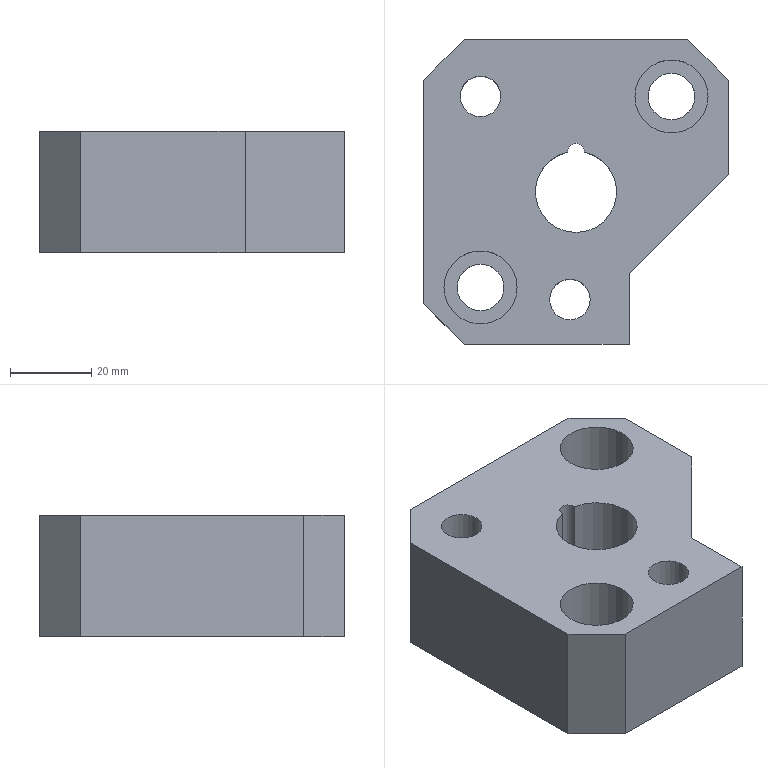Part | NX | features 23 2 | 1 solid | 21 faces | box 75 x 75 x 30 mm | volume 117467 mm3 | plane 13 | cylinder 8 | commonest cylinder face diameters 10.001 x2 11.5 x2 18 x2 4 x1 20 x1
STEP:
#1=CARTESIAN_POINT('',(80.528,385.45,-3.5));
#2=VERTEX_POINT('',#1);
#3=CARTESIAN_POINT('',(85.529,385.45,-3.5));
#4=DIRECTION('',(0.,0.,-1.));
#5=DIRECTION('',(-1.,0.,0.));
#6=AXIS2_PLACEMENT_3D('',#3,#4,#5);
#7=CIRCLE('',#6,5.);
#8=EDGE_CURVE('',#2,#2,#7,.T.);
#9=ORIENTED_EDGE('',*,*,#8,.F.);
#10=EDGE_LOOP('',(#9));
#11=FACE_BOUND('',#10,.T.);
#12=CARTESIAN_POINT('',(80.528,385.45,-33.5));
#13=VERTEX_POINT('',#12);
#14=CARTESIAN_POINT('',(85.529,385.45,-33.5));
#15=DIRECTION('',(0.,0.,-1.));
#16=DIRECTION('',(-1.,0.,0.));
#17=AXIS2_PLACEMENT_3D('',#14,#15,#16);
#18=CIRCLE('',#17,5.);
#19=EDGE_CURVE('',#13,#13,#18,.T.);
#20=ORIENTED_EDGE('',*,*,#19,.T.);
#21=EDGE_LOOP('',(#20));
#22=FACE_BOUND('',#21,.T.);
#23=CARTESIAN_POINT('',(85.529,385.45,198.5));
#24=DIRECTION('',(0.,0.,-1.));
#25=DIRECTION('',(0.,-1.,0.));
#26=AXIS2_PLACEMENT_3D('',#23,#24,#25);
#27=CYLINDRICAL_SURFACE('',#26,5.);
#28=ADVANCED_FACE('',(#11,#22),#27,.F.);
#29=CARTESIAN_POINT('',(104.779,435.45,-18.5));
#30=VERTEX_POINT('',#29);
#31=CARTESIAN_POINT('',(110.529,435.45,-18.5));
#32=DIRECTION('',(0.,0.,-1.));
#33=DIRECTION('',(-1.,0.,0.));
#34=AXIS2_PLACEMENT_3D('',#31,#32,#33);
#35=CIRCLE('',#34,5.75);
#36=EDGE_CURVE('',#30,#30,#35,.T.);
#37=ORIENTED_EDGE('',*,*,#36,.T.);
#38=EDGE_LOOP('',(#37));
#39=FACE_BOUND('',#38,.T.);
#40=CARTESIAN_POINT('',(101.529,435.45,-18.5));
#41=VERTEX_POINT('',#40);
#42=CARTESIAN_POINT('',(110.529,435.45,-18.5));
#43=DIRECTION('',(0.,0.,-1.));
#44=DIRECTION('',(-1.,0.,0.));
#45=AXIS2_PLACEMENT_3D('',#42,#43,#44);
#46=CIRCLE('',#45,9.);
#47=EDGE_CURVE('',#41,#41,#46,.T.);
#48=ORIENTED_EDGE('',*,*,#47,.F.);
#49=EDGE_LOOP('',(#48));
#50=FACE_BOUND('',#49,.T.);
#51=CARTESIAN_POINT('',(110.529,435.45,-18.5));
#52=DIRECTION('',(0.,0.,-1.));
#53=DIRECTION('',(0.,-1.,0.));
#54=AXIS2_PLACEMENT_3D('',#51,#52,#53);
#55=PLANE('',#54);
#56=ADVANCED_FACE('',(#39,#50),#55,.F.);
#57=CARTESIAN_POINT('',(57.779,388.45,-18.5));
#58=VERTEX_POINT('',#57);
#59=CARTESIAN_POINT('',(63.529,388.45,-18.5));
#60=DIRECTION('',(0.,0.,-1.));
#61=DIRECTION('',(-1.,0.,0.));
#62=AXIS2_PLACEMENT_3D('',#59,#60,#61);
#63=CIRCLE('',#62,5.75);
#64=EDGE_CURVE('',#58,#58,#63,.T.);
#65=ORIENTED_EDGE('',*,*,#64,.T.);
#66=EDGE_LOOP('',(#65));
#67=FACE_BOUND('',#66,.T.);
#68=CARTESIAN_POINT('',(54.529,388.45,-18.5));
#69=VERTEX_POINT('',#68);
#70=CARTESIAN_POINT('',(63.529,388.45,-18.5));
#71=DIRECTION('',(0.,0.,-1.));
#72=DIRECTION('',(-1.,0.,0.));
#73=AXIS2_PLACEMENT_3D('',#70,#71,#72);
#74=CIRCLE('',#73,9.);
#75=EDGE_CURVE('',#69,#69,#74,.T.);
#76=ORIENTED_EDGE('',*,*,#75,.F.);
#77=EDGE_LOOP('',(#76));
#78=FACE_BOUND('',#77,.T.);
#79=CARTESIAN_POINT('',(63.529,388.45,-18.5));
#80=DIRECTION('',(0.,0.,-1.));
#81=DIRECTION('',(0.,-1.,0.));
#82=AXIS2_PLACEMENT_3D('',#79,#80,#81);
#83=PLANE('',#82);
#84=ADVANCED_FACE('',(#67,#78),#83,.F.);
#85=CARTESIAN_POINT('',(104.779,435.45,-33.5));
#86=VERTEX_POINT('',#85);
#87=CARTESIAN_POINT('',(110.529,435.45,-33.5));
#88=DIRECTION('',(0.,0.,-1.));
#89=DIRECTION('',(-1.,0.,0.));
#90=AXIS2_PLACEMENT_3D('',#87,#88,#89);
#91=CIRCLE('',#90,5.75);
#92=EDGE_CURVE('',#86,#86,#91,.T.);
#93=ORIENTED_EDGE('',*,*,#92,.T.);
#94=EDGE_LOOP('',(#93));
#95=FACE_BOUND('',#94,.T.);
#96=ORIENTED_EDGE('',*,*,#36,.F.);
#97=EDGE_LOOP('',(#96));
#98=FACE_BOUND('',#97,.T.);
#99=CARTESIAN_POINT('',(110.529,435.45,-1.5));
#100=DIRECTION('',(0.,0.,-1.));
#101=DIRECTION('',(0.,1.,0.));
#102=AXIS2_PLACEMENT_3D('',#99,#100,#101);
#103=CYLINDRICAL_SURFACE('',#102,5.75);
#104=ADVANCED_FACE('',(#95,#98),#103,.F.);
#105=CARTESIAN_POINT('',(57.779,388.45,-33.5));
#106=VERTEX_POINT('',#105);
#107=CARTESIAN_POINT('',(63.529,388.45,-33.5));
#108=DIRECTION('',(0.,0.,-1.));
#109=DIRECTION('',(-1.,0.,0.));
#110=AXIS2_PLACEMENT_3D('',#107,#108,#109);
#111=CIRCLE('',#110,5.75);
#112=EDGE_CURVE('',#106,#106,#111,.T.);
#113=ORIENTED_EDGE('',*,*,#112,.T.);
#114=EDGE_LOOP('',(#113));
#115=FACE_BOUND('',#114,.T.);
#116=ORIENTED_EDGE('',*,*,#64,.F.);
#117=EDGE_LOOP('',(#116));
#118=FACE_BOUND('',#117,.T.);
#119=CARTESIAN_POINT('',(63.529,388.45,-1.5));
#120=DIRECTION('',(0.,0.,-1.));
#121=DIRECTION('',(0.,1.,0.));
#122=AXIS2_PLACEMENT_3D('',#119,#120,#121);
#123=CYLINDRICAL_SURFACE('',#122,5.75);
#124=ADVANCED_FACE('',(#115,#118),#123,.F.);
#125=ORIENTED_EDGE('',*,*,#47,.T.);
#126=EDGE_LOOP('',(#125));
#127=FACE_BOUND('',#126,.T.);
#128=CARTESIAN_POINT('',(101.529,435.45,-3.5));
#129=VERTEX_POINT('',#128);
#130=CARTESIAN_POINT('',(110.529,435.45,-3.5));
#131=DIRECTION('',(0.,0.,-1.));
#132=DIRECTION('',(-1.,0.,0.));
#133=AXIS2_PLACEMENT_3D('',#130,#131,#132);
#134=CIRCLE('',#133,9.);
#135=EDGE_CURVE('',#129,#129,#134,.T.);
#136=ORIENTED_EDGE('',*,*,#135,.F.);
#137=EDGE_LOOP('',(#136));
#138=FACE_BOUND('',#137,.T.);
#139=CARTESIAN_POINT('',(110.529,435.45,-3.5));
#140=DIRECTION('',(0.,0.,-1.));
#141=DIRECTION('',(0.,1.,0.));
#142=AXIS2_PLACEMENT_3D('',#139,#140,#141);
#143=CYLINDRICAL_SURFACE('',#142,9.);
#144=ADVANCED_FACE('',(#127,#138),#143,.F.);
#145=CARTESIAN_POINT('',(59.529,374.45,-33.5));
#146=VERTEX_POINT('',#145);
#147=CARTESIAN_POINT('',(49.529,384.45,-33.5));
#148=VERTEX_POINT('',#147);
#149=CARTESIAN_POINT('',(58.037,375.941,-33.5));
#150=DIRECTION('',(-0.7071,0.7071,0.));
#151=VECTOR('',#150,1000.);
#152=LINE('',#149,#151);
#153=EDGE_CURVE('',#146,#148,#152,.T.);
#154=ORIENTED_EDGE('',*,*,#153,.F.);
#155=CARTESIAN_POINT('',(59.529,374.45,-3.5));
#156=VERTEX_POINT('',#155);
#157=CARTESIAN_POINT('',(59.529,374.45,-23.5));
#158=DIRECTION('',(0.,0.,-1.));
#159=VECTOR('',#158,1000.);
#160=LINE('',#157,#159);
#161=EDGE_CURVE('',#156,#146,#160,.T.);
#162=ORIENTED_EDGE('',*,*,#161,.F.);
#163=CARTESIAN_POINT('',(49.529,384.45,-3.5));
#164=VERTEX_POINT('',#163);
#165=CARTESIAN_POINT('',(49.155,384.824,-3.5));
#166=DIRECTION('',(0.7071,-0.7071,0.));
#167=VECTOR('',#166,1000.);
#168=LINE('',#165,#167);
#169=EDGE_CURVE('',#164,#156,#168,.T.);
#170=ORIENTED_EDGE('',*,*,#169,.F.);
#171=CARTESIAN_POINT('',(49.529,384.45,-23.5));
#172=DIRECTION('',(0.,0.,1.));
#173=VECTOR('',#172,1000.);
#174=LINE('',#171,#173);
#175=EDGE_CURVE('',#148,#164,#174,.T.);
#176=ORIENTED_EDGE('',*,*,#175,.F.);
#177=EDGE_LOOP('',(#154,#162,#170,#176));
#178=FACE_BOUND('',#177,.T.);
#179=CARTESIAN_POINT('',(54.529,379.45,-23.5));
#180=DIRECTION('',(0.7071,0.7071,0.));
#181=DIRECTION('',(0.,0.,1.));
#182=AXIS2_PLACEMENT_3D('',#179,#180,#181);
#183=PLANE('',#182);
#184=ADVANCED_FACE('',(#178),#183,.F.);
#185=CARTESIAN_POINT('',(49.529,439.45,-3.5));
#186=VERTEX_POINT('',#185);
#187=CARTESIAN_POINT('',(49.529,411.95,-3.5));
#188=DIRECTION('',(0.,1.,0.));
#189=VECTOR('',#188,1000.);
#190=LINE('',#187,#189);
#191=EDGE_CURVE('',#164,#186,#190,.T.);
#192=ORIENTED_EDGE('',*,*,#191,.T.);
#193=CARTESIAN_POINT('',(49.529,439.45,-33.5));
#194=VERTEX_POINT('',#193);
#195=CARTESIAN_POINT('',(49.529,439.45,-23.5));
#196=DIRECTION('',(0.,0.,-1.));
#197=VECTOR('',#196,1000.);
#198=LINE('',#195,#197);
#199=EDGE_CURVE('',#186,#194,#198,.T.);
#200=ORIENTED_EDGE('',*,*,#199,.T.);
#201=CARTESIAN_POINT('',(49.529,411.95,-33.5));
#202=DIRECTION('',(0.,-1.,0.));
#203=VECTOR('',#202,1000.);
#204=LINE('',#201,#203);
#205=EDGE_CURVE('',#194,#148,#204,.T.);
#206=ORIENTED_EDGE('',*,*,#205,.T.);
#207=ORIENTED_EDGE('',*,*,#175,.T.);
#208=EDGE_LOOP('',(#192,#200,#206,#207));
#209=FACE_BOUND('',#208,.T.);
#210=CARTESIAN_POINT('',(49.529,411.95,-23.5));
#211=DIRECTION('',(-1.,0.,0.));
#212=DIRECTION('',(0.,0.,1.));
#213=AXIS2_PLACEMENT_3D('',#210,#211,#212);
#214=PLANE('',#213);
#215=ADVANCED_FACE('',(#209),#214,.T.);
#216=CARTESIAN_POINT('',(59.529,449.45,-33.5));
#217=VERTEX_POINT('',#216);
#218=CARTESIAN_POINT('',(85.464,475.385,-33.5));
#219=DIRECTION('',(0.7071,0.7071,0.));
#220=VECTOR('',#219,1000.);
#221=LINE('',#218,#220);
#222=EDGE_CURVE('',#194,#217,#221,.T.);
#223=ORIENTED_EDGE('',*,*,#222,.F.);
#224=ORIENTED_EDGE('',*,*,#199,.F.);
#225=CARTESIAN_POINT('',(59.529,449.45,-3.5));
#226=VERTEX_POINT('',#225);
#227=CARTESIAN_POINT('',(37.227,427.148,-3.5));
#228=DIRECTION('',(-0.7071,-0.7071,0.));
#229=VECTOR('',#228,1000.);
#230=LINE('',#227,#229);
#231=EDGE_CURVE('',#226,#186,#230,.T.);
#232=ORIENTED_EDGE('',*,*,#231,.F.);
#233=CARTESIAN_POINT('',(59.529,449.45,-23.5));
#234=DIRECTION('',(0.,0.,1.));
#235=VECTOR('',#234,1000.);
#236=LINE('',#233,#235);
#237=EDGE_CURVE('',#217,#226,#236,.T.);
#238=ORIENTED_EDGE('',*,*,#237,.F.);
#239=EDGE_LOOP('',(#223,#224,#232,#238));
#240=FACE_BOUND('',#239,.T.);
#241=CARTESIAN_POINT('',(54.529,444.45,-23.5));
#242=DIRECTION('',(0.7071,-0.7071,0.));
#243=DIRECTION('',(0.,0.,1.));
#244=AXIS2_PLACEMENT_3D('',#241,#242,#243);
#245=PLANE('',#244);
#246=ADVANCED_FACE('',(#240),#245,.F.);
#247=CARTESIAN_POINT('',(114.529,449.45,-3.5));
#248=VERTEX_POINT('',#247);
#249=CARTESIAN_POINT('',(87.029,449.45,-3.5));
#250=DIRECTION('',(1.,0.,0.));
#251=VECTOR('',#250,1000.);
#252=LINE('',#249,#251);
#253=EDGE_CURVE('',#226,#248,#252,.T.);
#254=ORIENTED_EDGE('',*,*,#253,.T.);
#255=CARTESIAN_POINT('',(114.529,449.45,-33.5));
#256=VERTEX_POINT('',#255);
#257=CARTESIAN_POINT('',(114.529,449.45,-23.5));
#258=DIRECTION('',(0.,0.,-1.));
#259=VECTOR('',#258,1000.);
#260=LINE('',#257,#259);
#261=EDGE_CURVE('',#248,#256,#260,.T.);
#262=ORIENTED_EDGE('',*,*,#261,.T.);
#263=CARTESIAN_POINT('',(87.029,449.45,-33.5));
#264=DIRECTION('',(-1.,0.,0.));
#265=VECTOR('',#264,1000.);
#266=LINE('',#263,#265);
#267=EDGE_CURVE('',#256,#217,#266,.T.);
#268=ORIENTED_EDGE('',*,*,#267,.T.);
#269=ORIENTED_EDGE('',*,*,#237,.T.);
#270=EDGE_LOOP('',(#254,#262,#268,#269));
#271=FACE_BOUND('',#270,.T.);
#272=CARTESIAN_POINT('',(87.029,449.45,-23.5));
#273=DIRECTION('',(0.,1.,0.));
#274=DIRECTION('',(0.,0.,-1.));
#275=AXIS2_PLACEMENT_3D('',#272,#273,#274);
#276=PLANE('',#275);
#277=ADVANCED_FACE('',(#271),#276,.T.);
#278=CARTESIAN_POINT('',(124.529,439.45,-33.5));
#279=VERTEX_POINT('',#278);
#280=CARTESIAN_POINT('',(123.037,440.941,-33.5));
#281=DIRECTION('',(0.7071,-0.7071,0.));
#282=VECTOR('',#281,1000.);
#283=LINE('',#280,#282);
#284=EDGE_CURVE('',#256,#279,#283,.T.);
#285=ORIENTED_EDGE('',*,*,#284,.F.);
#286=ORIENTED_EDGE('',*,*,#261,.F.);
#287=CARTESIAN_POINT('',(124.529,439.45,-3.5));
#288=VERTEX_POINT('',#287);
#289=CARTESIAN_POINT('',(114.155,449.824,-3.5));
#290=DIRECTION('',(-0.7071,0.7071,0.));
#291=VECTOR('',#290,1000.);
#292=LINE('',#289,#291);
#293=EDGE_CURVE('',#288,#248,#292,.T.);
#294=ORIENTED_EDGE('',*,*,#293,.F.);
#295=CARTESIAN_POINT('',(124.529,439.45,-23.5));
#296=DIRECTION('',(0.,0.,1.));
#297=VECTOR('',#296,1000.);
#298=LINE('',#295,#297);
#299=EDGE_CURVE('',#279,#288,#298,.T.);
#300=ORIENTED_EDGE('',*,*,#299,.F.);
#301=EDGE_LOOP('',(#285,#286,#294,#300));
#302=FACE_BOUND('',#301,.T.);
#303=CARTESIAN_POINT('',(124.529,439.45,-23.5));
#304=DIRECTION('',(-0.7071,-0.7071,0.));
#305=DIRECTION('',(0.,0.,1.));
#306=AXIS2_PLACEMENT_3D('',#303,#304,#305);
#307=PLANE('',#306);
#308=ADVANCED_FACE('',(#302),#307,.F.);
#309=CARTESIAN_POINT('',(124.529,416.278,-33.5));
#310=VERTEX_POINT('',#309);
#311=CARTESIAN_POINT('',(124.529,411.95,-33.5));
#312=DIRECTION('',(0.,1.,0.));
#313=VECTOR('',#312,1000.);
#314=LINE('',#311,#313);
#315=EDGE_CURVE('',#310,#279,#314,.T.);
#316=ORIENTED_EDGE('',*,*,#315,.T.);
#317=ORIENTED_EDGE('',*,*,#299,.T.);
#318=CARTESIAN_POINT('',(124.529,416.278,-3.5));
#319=VERTEX_POINT('',#318);
#320=CARTESIAN_POINT('',(124.529,411.95,-3.5));
#321=DIRECTION('',(0.,-1.,0.));
#322=VECTOR('',#321,1000.);
#323=LINE('',#320,#322);
#324=EDGE_CURVE('',#288,#319,#323,.T.);
#325=ORIENTED_EDGE('',*,*,#324,.T.);
#326=CARTESIAN_POINT('',(124.529,416.278,-23.5));
#327=DIRECTION('',(0.,0.,-1.));
#328=VECTOR('',#327,1000.);
#329=LINE('',#326,#328);
#330=EDGE_CURVE('',#319,#310,#329,.T.);
#331=ORIENTED_EDGE('',*,*,#330,.T.);
#332=EDGE_LOOP('',(#316,#317,#325,#331));
#333=FACE_BOUND('',#332,.T.);
#334=CARTESIAN_POINT('',(124.529,411.95,-23.5));
#335=DIRECTION('',(1.,0.,0.));
#336=DIRECTION('',(0.,0.,-1.));
#337=AXIS2_PLACEMENT_3D('',#334,#335,#336);
#338=PLANE('',#337);
#339=ADVANCED_FACE('',(#333),#338,.T.);
#340=CARTESIAN_POINT('',(100.109,391.859,-3.5));
#341=VERTEX_POINT('',#340);
#342=CARTESIAN_POINT('',(88.813,380.563,-3.5));
#343=DIRECTION('',(0.7071,0.7071,0.));
#344=VECTOR('',#343,1000.);
#345=LINE('',#342,#344);
#346=EDGE_CURVE('',#341,#319,#345,.T.);
#347=ORIENTED_EDGE('',*,*,#346,.F.);
#348=CARTESIAN_POINT('',(100.109,391.859,-33.5));
#349=VERTEX_POINT('',#348);
#350=CARTESIAN_POINT('',(100.109,391.859,-23.5));
#351=DIRECTION('',(0.,0.,-1.));
#352=VECTOR('',#351,1000.);
#353=LINE('',#350,#352);
#354=EDGE_CURVE('',#341,#349,#353,.T.);
#355=ORIENTED_EDGE('',*,*,#354,.T.);
#356=CARTESIAN_POINT('',(118.114,409.864,-33.5));
#357=DIRECTION('',(-0.7071,-0.7071,0.));
#358=VECTOR('',#357,1000.);
#359=LINE('',#356,#358);
#360=EDGE_CURVE('',#310,#349,#359,.T.);
#361=ORIENTED_EDGE('',*,*,#360,.F.);
#362=ORIENTED_EDGE('',*,*,#330,.F.);
#363=EDGE_LOOP('',(#347,#355,#361,#362));
#364=FACE_BOUND('',#363,.T.);
#365=CARTESIAN_POINT('',(118.114,409.864,-23.5));
#366=DIRECTION('',(-0.7071,0.7071,0.));
#367=DIRECTION('',(0.,0.,1.));
#368=AXIS2_PLACEMENT_3D('',#365,#366,#367);
#369=PLANE('',#368);
#370=ADVANCED_FACE('',(#364),#369,.F.);
#371=CARTESIAN_POINT('',(100.109,374.45,-33.5));
#372=VERTEX_POINT('',#371);
#373=CARTESIAN_POINT('',(100.109,444.376,-33.5));
#374=DIRECTION('',(0.,-1.,0.));
#375=VECTOR('',#374,1000.);
#376=LINE('',#373,#375);
#377=EDGE_CURVE('',#349,#372,#376,.T.);
#378=ORIENTED_EDGE('',*,*,#377,.F.);
#379=ORIENTED_EDGE('',*,*,#354,.F.);
#380=CARTESIAN_POINT('',(100.109,374.45,-3.5));
#381=VERTEX_POINT('',#380);
#382=CARTESIAN_POINT('',(100.109,392.723,-3.5));
#383=DIRECTION('',(0.,1.,0.));
#384=VECTOR('',#383,1000.);
#385=LINE('',#382,#384);
#386=EDGE_CURVE('',#381,#341,#385,.T.);
#387=ORIENTED_EDGE('',*,*,#386,.F.);
#388=CARTESIAN_POINT('',(100.109,374.45,-23.5));
#389=DIRECTION('',(0.,0.,1.));
#390=VECTOR('',#389,1000.);
#391=LINE('',#388,#390);
#392=EDGE_CURVE('',#372,#381,#391,.T.);
#393=ORIENTED_EDGE('',*,*,#392,.F.);
#394=EDGE_LOOP('',(#378,#379,#387,#393));
#395=FACE_BOUND('',#394,.T.);
#396=CARTESIAN_POINT('',(100.109,392.723,-8.5));
#397=DIRECTION('',(-1.,0.,0.));
#398=DIRECTION('',(0.,0.,1.));
#399=AXIS2_PLACEMENT_3D('',#396,#397,#398);
#400=PLANE('',#399);
#401=ADVANCED_FACE('',(#395),#400,.F.);
#402=CARTESIAN_POINT('',(87.029,374.45,-33.5));
#403=DIRECTION('',(1.,0.,0.));
#404=VECTOR('',#403,1000.);
#405=LINE('',#402,#404);
#406=EDGE_CURVE('',#146,#372,#405,.T.);
#407=ORIENTED_EDGE('',*,*,#406,.T.);
#408=ORIENTED_EDGE('',*,*,#392,.T.);
#409=CARTESIAN_POINT('',(87.029,374.45,-3.5));
#410=DIRECTION('',(-1.,0.,0.));
#411=VECTOR('',#410,1000.);
#412=LINE('',#409,#411);
#413=EDGE_CURVE('',#381,#156,#412,.T.);
#414=ORIENTED_EDGE('',*,*,#413,.T.);
#415=ORIENTED_EDGE('',*,*,#161,.T.);
#416=EDGE_LOOP('',(#407,#408,#414,#415));
#417=FACE_BOUND('',#416,.T.);
#418=CARTESIAN_POINT('',(87.029,374.45,-23.5));
#419=DIRECTION('',(0.,-1.,0.));
#420=DIRECTION('',(0.,0.,1.));
#421=AXIS2_PLACEMENT_3D('',#418,#419,#420);
#422=PLANE('',#421);
#423=ADVANCED_FACE('',(#417),#422,.T.);
#424=CARTESIAN_POINT('',(58.528,435.45,-3.5));
#425=VERTEX_POINT('',#424);
#426=CARTESIAN_POINT('',(63.529,435.45,-3.5));
#427=DIRECTION('',(0.,0.,1.));
#428=DIRECTION('',(-1.,0.,0.));
#429=AXIS2_PLACEMENT_3D('',#426,#427,#428);
#430=CIRCLE('',#429,5.);
#431=EDGE_CURVE('',#425,#425,#430,.T.);
#432=ORIENTED_EDGE('',*,*,#431,.T.);
#433=EDGE_LOOP('',(#432));
#434=FACE_BOUND('',#433,.T.);
#435=CARTESIAN_POINT('',(58.528,435.45,-33.5));
#436=VERTEX_POINT('',#435);
#437=CARTESIAN_POINT('',(63.529,435.45,-33.5));
#438=DIRECTION('',(0.,0.,-1.));
#439=DIRECTION('',(-1.,0.,0.));
#440=AXIS2_PLACEMENT_3D('',#437,#438,#439);
#441=CIRCLE('',#440,5.);
#442=EDGE_CURVE('',#436,#436,#441,.T.);
#443=ORIENTED_EDGE('',*,*,#442,.T.);
#444=EDGE_LOOP('',(#443));
#445=FACE_BOUND('',#444,.T.);
#446=CARTESIAN_POINT('',(63.529,435.45,198.5));
#447=DIRECTION('',(0.,0.,-1.));
#448=DIRECTION('',(0.,-1.,0.));
#449=AXIS2_PLACEMENT_3D('',#446,#447,#448);
#450=CYLINDRICAL_SURFACE('',#449,5.);
#451=ADVANCED_FACE('',(#434,#445),#450,.F.);
#452=ORIENTED_EDGE('',*,*,#75,.T.);
#453=EDGE_LOOP('',(#452));
#454=FACE_BOUND('',#453,.T.);
#455=CARTESIAN_POINT('',(54.529,388.45,-3.5));
#456=VERTEX_POINT('',#455);
#457=CARTESIAN_POINT('',(63.529,388.45,-3.5));
#458=DIRECTION('',(0.,0.,-1.));
#459=DIRECTION('',(-1.,0.,0.));
#460=AXIS2_PLACEMENT_3D('',#457,#458,#459);
#461=CIRCLE('',#460,9.);
#462=EDGE_CURVE('',#456,#456,#461,.T.);
#463=ORIENTED_EDGE('',*,*,#462,.F.);
#464=EDGE_LOOP('',(#463));
#465=FACE_BOUND('',#464,.T.);
#466=CARTESIAN_POINT('',(63.529,388.45,-3.5));
#467=DIRECTION('',(0.,0.,-1.));
#468=DIRECTION('',(0.,1.,0.));
#469=AXIS2_PLACEMENT_3D('',#466,#467,#468);
#470=CYLINDRICAL_SURFACE('',#469,9.);
#471=ADVANCED_FACE('',(#454,#465),#470,.F.);
#472=CARTESIAN_POINT('',(89.019,421.75,-33.5));
#473=VERTEX_POINT('',#472);
#474=CARTESIAN_POINT('',(85.039,421.75,-33.5));
#475=VERTEX_POINT('',#474);
#476=CARTESIAN_POINT('',(87.029,411.95,-33.5));
#477=DIRECTION('',(0.,0.,-1.));
#478=DIRECTION('',(-1.,0.,0.));
#479=AXIS2_PLACEMENT_3D('',#476,#477,#478);
#480=CIRCLE('',#479,10.);
#481=EDGE_CURVE('',#473,#475,#480,.T.);
#482=ORIENTED_EDGE('',*,*,#481,.T.);
#483=CARTESIAN_POINT('',(85.039,421.75,-3.5));
#484=VERTEX_POINT('',#483);
#485=CARTESIAN_POINT('',(85.039,421.75,-53.5));
#486=DIRECTION('',(0.,0.,1.));
#487=VECTOR('',#486,1000.);
#488=LINE('',#485,#487);
#489=EDGE_CURVE('',#475,#484,#488,.T.);
#490=ORIENTED_EDGE('',*,*,#489,.T.);
#491=CARTESIAN_POINT('',(89.019,421.75,-3.5));
#492=VERTEX_POINT('',#491);
#493=CARTESIAN_POINT('',(87.029,411.95,-3.5));
#494=DIRECTION('',(0.,0.,1.));
#495=DIRECTION('',(-1.,0.,0.));
#496=AXIS2_PLACEMENT_3D('',#493,#494,#495);
#497=CIRCLE('',#496,10.);
#498=EDGE_CURVE('',#484,#492,#497,.T.);
#499=ORIENTED_EDGE('',*,*,#498,.T.);
#500=CARTESIAN_POINT('',(89.019,421.75,-53.5));
#501=DIRECTION('',(0.,0.,-1.));
#502=VECTOR('',#501,1000.);
#503=LINE('',#500,#502);
#504=EDGE_CURVE('',#492,#473,#503,.T.);
#505=ORIENTED_EDGE('',*,*,#504,.T.);
#506=EDGE_LOOP('',(#482,#490,#499,#505));
#507=FACE_BOUND('',#506,.T.);
#508=CARTESIAN_POINT('',(87.029,411.95,-18.5));
#509=DIRECTION('',(0.,0.,1.));
#510=DIRECTION('',(1.,0.,0.));
#511=AXIS2_PLACEMENT_3D('',#508,#509,#510);
#512=CYLINDRICAL_SURFACE('',#511,10.);
#513=ADVANCED_FACE('',(#507),#512,.F.);
#514=ORIENTED_EDGE('',*,*,#8,.T.);
#515=EDGE_LOOP('',(#514));
#516=FACE_BOUND('',#515,.T.);
#517=ORIENTED_EDGE('',*,*,#498,.F.);
#518=CARTESIAN_POINT('',(87.029,421.95,-3.5));
#519=DIRECTION('',(0.,0.,-1.));
#520=DIRECTION('',(1.,0.,0.));
#521=AXIS2_PLACEMENT_3D('',#518,#519,#520);
#522=CIRCLE('',#521,2.);
#523=EDGE_CURVE('',#484,#492,#522,.T.);
#524=ORIENTED_EDGE('',*,*,#523,.T.);
#525=EDGE_LOOP('',(#517,#524));
#526=FACE_BOUND('',#525,.T.);
#527=ORIENTED_EDGE('',*,*,#462,.T.);
#528=EDGE_LOOP('',(#527));
#529=FACE_BOUND('',#528,.T.);
#530=ORIENTED_EDGE('',*,*,#431,.F.);
#531=EDGE_LOOP('',(#530));
#532=FACE_BOUND('',#531,.T.);
#533=ORIENTED_EDGE('',*,*,#413,.F.);
#534=ORIENTED_EDGE('',*,*,#386,.T.);
#535=ORIENTED_EDGE('',*,*,#346,.T.);
#536=ORIENTED_EDGE('',*,*,#324,.F.);
#537=ORIENTED_EDGE('',*,*,#293,.T.);
#538=ORIENTED_EDGE('',*,*,#253,.F.);
#539=ORIENTED_EDGE('',*,*,#231,.T.);
#540=ORIENTED_EDGE('',*,*,#191,.F.);
#541=ORIENTED_EDGE('',*,*,#169,.T.);
#542=EDGE_LOOP('',(#533,#534,#535,#536,#537,#538,#539,#540,#541));
#543=FACE_BOUND('',#542,.T.);
#544=ORIENTED_EDGE('',*,*,#135,.T.);
#545=EDGE_LOOP('',(#544));
#546=FACE_BOUND('',#545,.T.);
#547=CARTESIAN_POINT('',(64.353,405.022,-3.5));
#548=DIRECTION('',(0.,0.,-1.));
#549=DIRECTION('',(0.,-1.,0.));
#550=AXIS2_PLACEMENT_3D('',#547,#548,#549);
#551=PLANE('',#550);
#552=ADVANCED_FACE('',(#516,#526,#529,#532,#543,#546),#551,.F.);
#553=CARTESIAN_POINT('',(87.029,421.95,-33.5));
#554=DIRECTION('',(0.,0.,-1.));
#555=DIRECTION('',(-1.,0.,0.));
#556=AXIS2_PLACEMENT_3D('',#553,#554,#555);
#557=CIRCLE('',#556,2.);
#558=EDGE_CURVE('',#475,#473,#557,.T.);
#559=ORIENTED_EDGE('',*,*,#558,.F.);
#560=ORIENTED_EDGE('',*,*,#481,.F.);
#561=EDGE_LOOP('',(#559,#560));
#562=FACE_BOUND('',#561,.T.);
#563=ORIENTED_EDGE('',*,*,#19,.F.);
#564=EDGE_LOOP('',(#563));
#565=FACE_BOUND('',#564,.T.);
#566=ORIENTED_EDGE('',*,*,#112,.F.);
#567=EDGE_LOOP('',(#566));
#568=FACE_BOUND('',#567,.T.);
#569=ORIENTED_EDGE('',*,*,#442,.F.);
#570=EDGE_LOOP('',(#569));
#571=FACE_BOUND('',#570,.T.);
#572=ORIENTED_EDGE('',*,*,#92,.F.);
#573=EDGE_LOOP('',(#572));
#574=FACE_BOUND('',#573,.T.);
#575=ORIENTED_EDGE('',*,*,#360,.T.);
#576=ORIENTED_EDGE('',*,*,#377,.T.);
#577=ORIENTED_EDGE('',*,*,#406,.F.);
#578=ORIENTED_EDGE('',*,*,#153,.T.);
#579=ORIENTED_EDGE('',*,*,#205,.F.);
#580=ORIENTED_EDGE('',*,*,#222,.T.);
#581=ORIENTED_EDGE('',*,*,#267,.F.);
#582=ORIENTED_EDGE('',*,*,#284,.T.);
#583=ORIENTED_EDGE('',*,*,#315,.F.);
#584=EDGE_LOOP('',(#575,#576,#577,#578,#579,#580,#581,#582,#583));
#585=FACE_BOUND('',#584,.T.);
#586=CARTESIAN_POINT('',(121.472,444.376,-33.5));
#587=DIRECTION('',(0.,0.,-1.));
#588=DIRECTION('',(0.,-1.,0.));
#589=AXIS2_PLACEMENT_3D('',#586,#587,#588);
#590=PLANE('',#589);
#591=ADVANCED_FACE('',(#562,#565,#568,#571,#574,#585),#590,.T.);
#592=ORIENTED_EDGE('',*,*,#558,.T.);
#593=ORIENTED_EDGE('',*,*,#504,.F.);
#594=ORIENTED_EDGE('',*,*,#523,.F.);
#595=ORIENTED_EDGE('',*,*,#489,.F.);
#596=EDGE_LOOP('',(#592,#593,#594,#595));
#597=FACE_BOUND('',#596,.T.);
#598=CARTESIAN_POINT('',(87.029,421.95,-3.5));
#599=DIRECTION('',(0.,0.,-1.));
#600=DIRECTION('',(-1.,0.,0.));
#601=AXIS2_PLACEMENT_3D('',#598,#599,#600);
#602=CYLINDRICAL_SURFACE('',#601,2.);
#603=ADVANCED_FACE('',(#597),#602,.F.);
#604=CLOSED_SHELL('',(#28,#56,#84,#104,#124,#144,#184,#215,#246,#277,#308,#339,#370,#401,#423,#451,#471,#513,#552,#591,#603));
#605=MANIFOLD_SOLID_BREP('',#604);
#606=(LENGTH_UNIT()NAMED_UNIT(*)SI_UNIT(.MILLI.,.METRE.));
#607=UNCERTAINTY_MEASURE_WITH_UNIT(LENGTH_MEASURE(0.00001),#606,'','');
#608=(NAMED_UNIT(*)PLANE_ANGLE_UNIT()SI_UNIT($,.RADIAN.));
#609=(NAMED_UNIT(*)SI_UNIT($,.STERADIAN.)SOLID_ANGLE_UNIT());
#610=(GEOMETRIC_REPRESENTATION_CONTEXT(3)GLOBAL_UNCERTAINTY_ASSIGNED_CONTEXT((#607))GLOBAL_UNIT_ASSIGNED_CONTEXT((#606,#608,#609))REPRESENTATION_CONTEXT('',''));
#611=ADVANCED_BREP_SHAPE_REPRESENTATION('',(#605),#610);